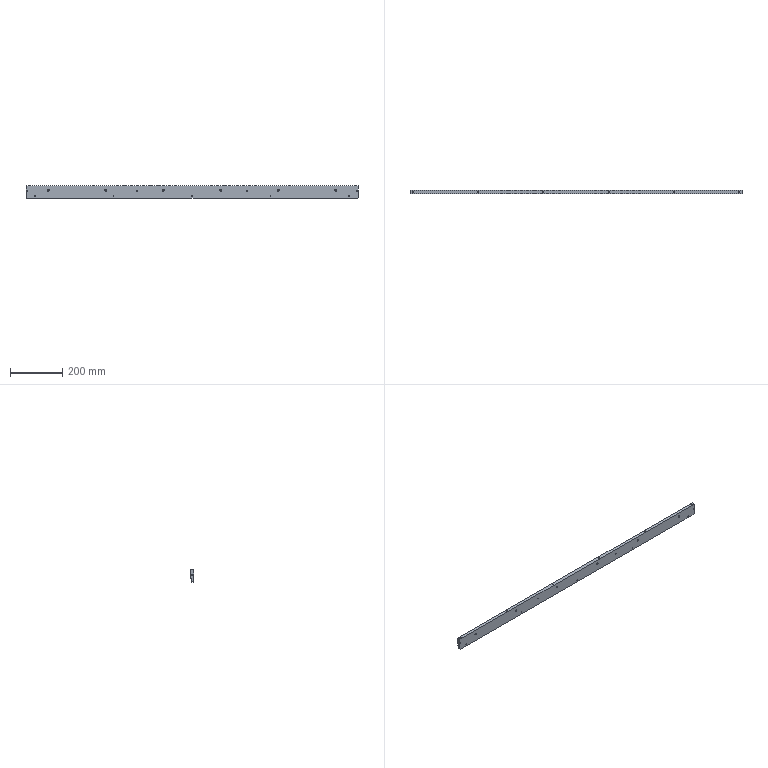Part | SolidWorks | features HoleWzd 4, ICE 2, Chamfer 1, Extrusion 1 | 1 solid | 82 faces | box 1270 x 12 x 47 mm | volume 615944 mm3 | cylinder 54 | plane 16 | cone 12 | commonest cylinder face diameters 4.2 x12 6.8 x12 10 x12 2.5 x10 3.3 x8